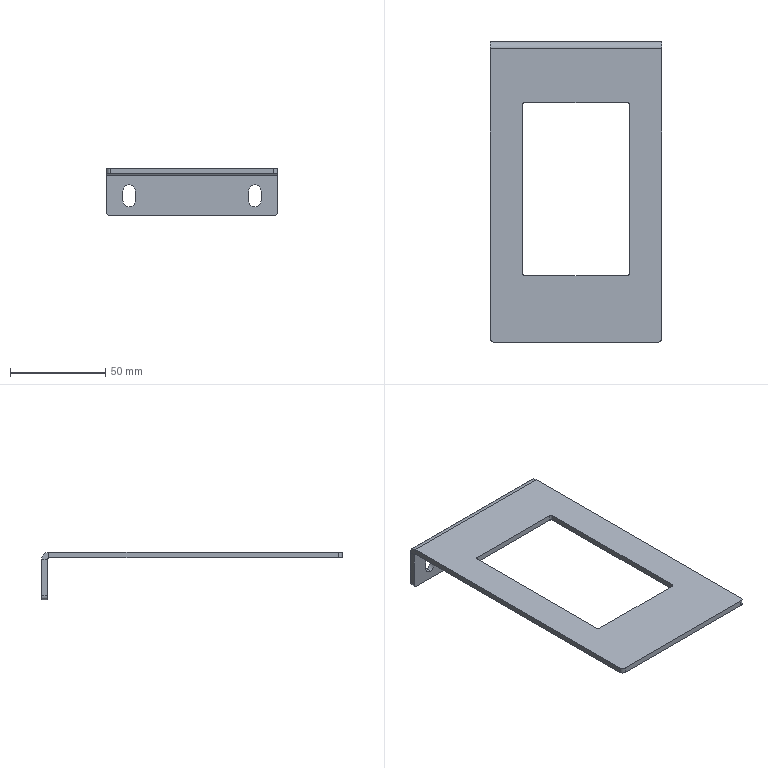Part | SolidWorks | features Fillet 2, ICE 2, EdgeFlange 1, FlatPattern 1, SMBaseFlange 1, SheetMetal 1 | 1 solid | 36 faces | box 90 x 158 x 25 mm | volume 32642 mm3 | plane 20 | cylinder 16 | commonest cylinder face diameters 6.6 x6 2 x4 4 x4 1.473 x1 7.473 x1
STEP:
#1=CARTESIAN_POINT('',(-33.,80.5,-20.3));
#2=VERTEX_POINT('',#1);
#3=CARTESIAN_POINT('',(-29.7,80.5,-17.));
#4=VERTEX_POINT('',#3);
#5=CARTESIAN_POINT('',(-33.,80.5,-17.));
#6=DIRECTION('',(0.,-1.,0.));
#7=DIRECTION('',(0.,0.,-1.));
#8=AXIS2_PLACEMENT_3D('',#5,#6,#7);
#9=CIRCLE('',#8,3.3);
#10=EDGE_CURVE('',#2,#4,#9,.T.);
#11=ORIENTED_EDGE('',*,*,#10,.F.);
#12=CARTESIAN_POINT('',(-33.,77.5,-20.3));
#13=VERTEX_POINT('',#12);
#14=CARTESIAN_POINT('',(-33.,80.5,-20.3));
#15=DIRECTION('',(0.,-1.,0.));
#16=VECTOR('',#15,1000.);
#17=LINE('',#14,#16);
#18=EDGE_CURVE('',#2,#13,#17,.T.);
#19=ORIENTED_EDGE('',*,*,#18,.T.);
#20=CARTESIAN_POINT('',(-29.7,77.5,-17.));
#21=VERTEX_POINT('',#20);
#22=CARTESIAN_POINT('',(-33.,77.5,-17.));
#23=DIRECTION('',(0.,-1.,0.));
#24=DIRECTION('',(0.,0.,-1.));
#25=AXIS2_PLACEMENT_3D('',#22,#23,#24);
#26=CIRCLE('',#25,3.3);
#27=EDGE_CURVE('',#13,#21,#26,.T.);
#28=ORIENTED_EDGE('',*,*,#27,.T.);
#29=CARTESIAN_POINT('',(-29.7,80.5,-17.));
#30=DIRECTION('',(0.,-1.,0.));
#31=VECTOR('',#30,1000.);
#32=LINE('',#29,#31);
#33=EDGE_CURVE('',#4,#21,#32,.T.);
#34=ORIENTED_EDGE('',*,*,#33,.F.);
#35=EDGE_LOOP('',(#11,#19,#28,#34));
#36=FACE_OUTER_BOUND('',#35,.T.);
#37=CARTESIAN_POINT('',(-33.,80.5,-17.));
#38=DIRECTION('',(0.,-1.,0.));
#39=DIRECTION('',(0.,0.,-1.));
#40=AXIS2_PLACEMENT_3D('',#37,#38,#39);
#41=CYLINDRICAL_SURFACE('',#40,3.3);
#42=ADVANCED_FACE('',(#36),#41,.F.);
#43=CARTESIAN_POINT('',(33.,80.5,-20.3));
#44=VERTEX_POINT('',#43);
#45=CARTESIAN_POINT('',(36.3,80.5,-17.));
#46=VERTEX_POINT('',#45);
#47=CARTESIAN_POINT('',(33.,80.5,-17.));
#48=DIRECTION('',(0.,-1.,0.));
#49=DIRECTION('',(0.,0.,-1.));
#50=AXIS2_PLACEMENT_3D('',#47,#48,#49);
#51=CIRCLE('',#50,3.3);
#52=EDGE_CURVE('',#44,#46,#51,.T.);
#53=ORIENTED_EDGE('',*,*,#52,.F.);
#54=CARTESIAN_POINT('',(33.,77.5,-20.3));
#55=VERTEX_POINT('',#54);
#56=CARTESIAN_POINT('',(33.,80.5,-20.3));
#57=DIRECTION('',(0.,-1.,0.));
#58=VECTOR('',#57,1000.);
#59=LINE('',#56,#58);
#60=EDGE_CURVE('',#44,#55,#59,.T.);
#61=ORIENTED_EDGE('',*,*,#60,.T.);
#62=CARTESIAN_POINT('',(36.3,77.5,-17.));
#63=VERTEX_POINT('',#62);
#64=CARTESIAN_POINT('',(33.,77.5,-17.));
#65=DIRECTION('',(0.,-1.,0.));
#66=DIRECTION('',(0.,0.,-1.));
#67=AXIS2_PLACEMENT_3D('',#64,#65,#66);
#68=CIRCLE('',#67,3.3);
#69=EDGE_CURVE('',#55,#63,#68,.T.);
#70=ORIENTED_EDGE('',*,*,#69,.T.);
#71=CARTESIAN_POINT('',(36.3,80.5,-17.));
#72=DIRECTION('',(0.,-1.,0.));
#73=VECTOR('',#72,1000.);
#74=LINE('',#71,#73);
#75=EDGE_CURVE('',#46,#63,#74,.T.);
#76=ORIENTED_EDGE('',*,*,#75,.F.);
#77=EDGE_LOOP('',(#53,#61,#70,#76));
#78=FACE_OUTER_BOUND('',#77,.T.);
#79=CARTESIAN_POINT('',(33.,80.5,-17.));
#80=DIRECTION('',(0.,-1.,0.));
#81=DIRECTION('',(0.,0.,-1.));
#82=AXIS2_PLACEMENT_3D('',#79,#80,#81);
#83=CYLINDRICAL_SURFACE('',#82,3.3);
#84=ADVANCED_FACE('',(#78),#83,.F.);
#85=CARTESIAN_POINT('',(45.,-75.5,0.));
#86=VERTEX_POINT('',#85);
#87=CARTESIAN_POINT('',(45.,76.763,0.));
#88=VERTEX_POINT('',#87);
#89=CARTESIAN_POINT('',(45.,77.5,0.));
#90=DIRECTION('',(0.,1.,0.));
#91=VECTOR('',#90,1000.);
#92=LINE('',#89,#91);
#93=EDGE_CURVE('',#86,#88,#92,.T.);
#94=ORIENTED_EDGE('',*,*,#93,.F.);
#95=CARTESIAN_POINT('',(45.,-75.5,-3.));
#96=VERTEX_POINT('',#95);
#97=CARTESIAN_POINT('',(45.,-75.5,-3.));
#98=DIRECTION('',(0.,0.,-1.));
#99=VECTOR('',#98,1000.);
#100=LINE('',#97,#99);
#101=EDGE_CURVE('',#86,#96,#100,.T.);
#102=ORIENTED_EDGE('',*,*,#101,.T.);
#103=CARTESIAN_POINT('',(45.,76.763,-3.));
#104=VERTEX_POINT('',#103);
#105=CARTESIAN_POINT('',(45.,77.5,-3.));
#106=DIRECTION('',(0.,1.,0.));
#107=VECTOR('',#106,1000.);
#108=LINE('',#105,#107);
#109=EDGE_CURVE('',#96,#104,#108,.T.);
#110=ORIENTED_EDGE('',*,*,#109,.T.);
#111=CARTESIAN_POINT('',(45.,76.763,-3.));
#112=DIRECTION('',(0.,0.,1.));
#113=VECTOR('',#112,1000.);
#114=LINE('',#111,#113);
#115=EDGE_CURVE('',#104,#88,#114,.T.);
#116=ORIENTED_EDGE('',*,*,#115,.T.);
#117=EDGE_LOOP('',(#94,#102,#110,#116));
#118=FACE_OUTER_BOUND('',#117,.T.);
#119=CARTESIAN_POINT('',(45.,77.5,-3.));
#120=DIRECTION('',(1.,0.,0.));
#121=DIRECTION('',(0.,1.,0.));
#122=AXIS2_PLACEMENT_3D('',#119,#120,#121);
#123=PLANE('',#122);
#124=ADVANCED_FACE('',(#118),#123,.T.);
#125=CARTESIAN_POINT('',(-27.,48.5,-3.));
#126=VERTEX_POINT('',#125);
#127=CARTESIAN_POINT('',(27.,48.5,-3.));
#128=VERTEX_POINT('',#127);
#129=CARTESIAN_POINT('',(28.,48.5,-3.));
#130=DIRECTION('',(1.,0.,0.));
#131=VECTOR('',#130,1000.);
#132=LINE('',#129,#131);
#133=EDGE_CURVE('',#126,#128,#132,.T.);
#134=ORIENTED_EDGE('',*,*,#133,.F.);
#135=CARTESIAN_POINT('',(-28.,47.5,-3.));
#136=VERTEX_POINT('',#135);
#137=CARTESIAN_POINT('',(-27.,47.5,-3.));
#138=DIRECTION('',(0.,0.,1.));
#139=DIRECTION('',(1.,0.,0.));
#140=AXIS2_PLACEMENT_3D('',#137,#138,#139);
#141=CIRCLE('',#140,1.);
#142=EDGE_CURVE('',#126,#136,#141,.T.);
#143=ORIENTED_EDGE('',*,*,#142,.T.);
#144=CARTESIAN_POINT('',(-28.,-41.5,-3.));
#145=VERTEX_POINT('',#144);
#146=CARTESIAN_POINT('',(-28.,-42.5,-3.));
#147=DIRECTION('',(0.,1.,0.));
#148=VECTOR('',#147,1000.);
#149=LINE('',#146,#148);
#150=EDGE_CURVE('',#145,#136,#149,.T.);
#151=ORIENTED_EDGE('',*,*,#150,.F.);
#152=CARTESIAN_POINT('',(-27.,-42.5,-3.));
#153=VERTEX_POINT('',#152);
#154=CARTESIAN_POINT('',(-27.,-41.5,-3.));
#155=DIRECTION('',(0.,0.,1.));
#156=DIRECTION('',(1.,0.,0.));
#157=AXIS2_PLACEMENT_3D('',#154,#155,#156);
#158=CIRCLE('',#157,1.);
#159=EDGE_CURVE('',#145,#153,#158,.T.);
#160=ORIENTED_EDGE('',*,*,#159,.T.);
#161=CARTESIAN_POINT('',(27.,-42.5,-3.));
#162=VERTEX_POINT('',#161);
#163=CARTESIAN_POINT('',(28.,-42.5,-3.));
#164=DIRECTION('',(-1.,0.,0.));
#165=VECTOR('',#164,1000.);
#166=LINE('',#163,#165);
#167=EDGE_CURVE('',#162,#153,#166,.T.);
#168=ORIENTED_EDGE('',*,*,#167,.F.);
#169=CARTESIAN_POINT('',(28.,-41.5,-3.));
#170=VERTEX_POINT('',#169);
#171=CARTESIAN_POINT('',(27.,-41.5,-3.));
#172=DIRECTION('',(0.,0.,1.));
#173=DIRECTION('',(1.,0.,0.));
#174=AXIS2_PLACEMENT_3D('',#171,#172,#173);
#175=CIRCLE('',#174,1.);
#176=EDGE_CURVE('',#162,#170,#175,.T.);
#177=ORIENTED_EDGE('',*,*,#176,.T.);
#178=CARTESIAN_POINT('',(28.,47.5,-3.));
#179=VERTEX_POINT('',#178);
#180=CARTESIAN_POINT('',(28.,-42.5,-3.));
#181=DIRECTION('',(0.,-1.,0.));
#182=VECTOR('',#181,1000.);
#183=LINE('',#180,#182);
#184=EDGE_CURVE('',#179,#170,#183,.T.);
#185=ORIENTED_EDGE('',*,*,#184,.F.);
#186=CARTESIAN_POINT('',(27.,47.5,-3.));
#187=DIRECTION('',(0.,0.,1.));
#188=DIRECTION('',(1.,0.,0.));
#189=AXIS2_PLACEMENT_3D('',#186,#187,#188);
#190=CIRCLE('',#189,1.);
#191=EDGE_CURVE('',#179,#128,#190,.T.);
#192=ORIENTED_EDGE('',*,*,#191,.T.);
#193=EDGE_LOOP('',(#134,#143,#151,#160,#168,#177,#185,#192));
#194=FACE_BOUND('',#193,.T.);
#195=CARTESIAN_POINT('',(-43.,-77.5,-3.));
#196=VERTEX_POINT('',#195);
#197=CARTESIAN_POINT('',(43.,-77.5,-3.));
#198=VERTEX_POINT('',#197);
#199=CARTESIAN_POINT('',(-45.,-77.5,-3.));
#200=DIRECTION('',(1.,0.,0.));
#201=VECTOR('',#200,1000.);
#202=LINE('',#199,#201);
#203=EDGE_CURVE('',#196,#198,#202,.T.);
#204=ORIENTED_EDGE('',*,*,#203,.F.);
#205=CARTESIAN_POINT('',(-45.,-75.5,-3.));
#206=VERTEX_POINT('',#205);
#207=CARTESIAN_POINT('',(-43.,-75.5,-3.));
#208=DIRECTION('',(0.,0.,-1.));
#209=DIRECTION('',(1.,0.,0.));
#210=AXIS2_PLACEMENT_3D('',#207,#208,#209);
#211=CIRCLE('',#210,2.);
#212=EDGE_CURVE('',#196,#206,#211,.T.);
#213=ORIENTED_EDGE('',*,*,#212,.T.);
#214=CARTESIAN_POINT('',(-45.,76.763,-3.));
#215=VERTEX_POINT('',#214);
#216=CARTESIAN_POINT('',(-45.,77.5,-3.));
#217=DIRECTION('',(0.,-1.,0.));
#218=VECTOR('',#217,1000.);
#219=LINE('',#216,#218);
#220=EDGE_CURVE('',#215,#206,#219,.T.);
#221=ORIENTED_EDGE('',*,*,#220,.F.);
#222=CARTESIAN_POINT('',(45.,76.763,-3.));
#223=DIRECTION('',(-1.,0.,0.));
#224=VECTOR('',#223,1000.);
#225=LINE('',#222,#224);
#226=EDGE_CURVE('',#104,#215,#225,.T.);
#227=ORIENTED_EDGE('',*,*,#226,.F.);
#228=ORIENTED_EDGE('',*,*,#109,.F.);
#229=CARTESIAN_POINT('',(43.,-75.5,-3.));
#230=DIRECTION('',(0.,0.,-1.));
#231=DIRECTION('',(1.,0.,0.));
#232=AXIS2_PLACEMENT_3D('',#229,#230,#231);
#233=CIRCLE('',#232,2.);
#234=EDGE_CURVE('',#96,#198,#233,.T.);
#235=ORIENTED_EDGE('',*,*,#234,.T.);
#236=EDGE_LOOP('',(#204,#213,#221,#227,#228,#235));
#237=FACE_OUTER_BOUND('',#236,.T.);
#238=CARTESIAN_POINT('',(45.,-77.5,-3.));
#239=DIRECTION('',(0.,0.,1.));
#240=DIRECTION('',(1.,0.,0.));
#241=AXIS2_PLACEMENT_3D('',#238,#239,#240);
#242=PLANE('',#241);
#243=ADVANCED_FACE('',(#194,#237),#242,.F.);
#244=CARTESIAN_POINT('',(27.,-42.5,0.));
#245=VERTEX_POINT('',#244);
#246=CARTESIAN_POINT('',(-27.,-42.5,0.));
#247=VERTEX_POINT('',#246);
#248=CARTESIAN_POINT('',(28.,-42.5,0.));
#249=DIRECTION('',(-1.,0.,0.));
#250=VECTOR('',#249,1000.);
#251=LINE('',#248,#250);
#252=EDGE_CURVE('',#245,#247,#251,.T.);
#253=ORIENTED_EDGE('',*,*,#252,.T.);
#254=CARTESIAN_POINT('',(-28.,-41.5,0.));
#255=VERTEX_POINT('',#254);
#256=CARTESIAN_POINT('',(-27.,-41.5,0.));
#257=DIRECTION('',(0.,0.,-1.));
#258=DIRECTION('',(1.,0.,0.));
#259=AXIS2_PLACEMENT_3D('',#256,#257,#258);
#260=CIRCLE('',#259,1.);
#261=EDGE_CURVE('',#247,#255,#260,.T.);
#262=ORIENTED_EDGE('',*,*,#261,.T.);
#263=CARTESIAN_POINT('',(-28.,47.5,0.));
#264=VERTEX_POINT('',#263);
#265=CARTESIAN_POINT('',(-28.,-42.5,0.));
#266=DIRECTION('',(0.,1.,0.));
#267=VECTOR('',#266,1000.);
#268=LINE('',#265,#267);
#269=EDGE_CURVE('',#255,#264,#268,.T.);
#270=ORIENTED_EDGE('',*,*,#269,.T.);
#271=CARTESIAN_POINT('',(-27.,48.5,0.));
#272=VERTEX_POINT('',#271);
#273=CARTESIAN_POINT('',(-27.,47.5,0.));
#274=DIRECTION('',(0.,0.,-1.));
#275=DIRECTION('',(1.,0.,0.));
#276=AXIS2_PLACEMENT_3D('',#273,#274,#275);
#277=CIRCLE('',#276,1.);
#278=EDGE_CURVE('',#264,#272,#277,.T.);
#279=ORIENTED_EDGE('',*,*,#278,.T.);
#280=CARTESIAN_POINT('',(27.,48.5,0.));
#281=VERTEX_POINT('',#280);
#282=CARTESIAN_POINT('',(28.,48.5,0.));
#283=DIRECTION('',(1.,0.,0.));
#284=VECTOR('',#283,1000.);
#285=LINE('',#282,#284);
#286=EDGE_CURVE('',#272,#281,#285,.T.);
#287=ORIENTED_EDGE('',*,*,#286,.T.);
#288=CARTESIAN_POINT('',(28.,47.5,0.));
#289=VERTEX_POINT('',#288);
#290=CARTESIAN_POINT('',(27.,47.5,0.));
#291=DIRECTION('',(0.,0.,-1.));
#292=DIRECTION('',(1.,0.,0.));
#293=AXIS2_PLACEMENT_3D('',#290,#291,#292);
#294=CIRCLE('',#293,1.);
#295=EDGE_CURVE('',#281,#289,#294,.T.);
#296=ORIENTED_EDGE('',*,*,#295,.T.);
#297=CARTESIAN_POINT('',(28.,-41.5,0.));
#298=VERTEX_POINT('',#297);
#299=CARTESIAN_POINT('',(28.,-42.5,0.));
#300=DIRECTION('',(0.,-1.,0.));
#301=VECTOR('',#300,1000.);
#302=LINE('',#299,#301);
#303=EDGE_CURVE('',#289,#298,#302,.T.);
#304=ORIENTED_EDGE('',*,*,#303,.T.);
#305=CARTESIAN_POINT('',(27.,-41.5,0.));
#306=DIRECTION('',(0.,0.,-1.));
#307=DIRECTION('',(1.,0.,0.));
#308=AXIS2_PLACEMENT_3D('',#305,#306,#307);
#309=CIRCLE('',#308,1.);
#310=EDGE_CURVE('',#298,#245,#309,.T.);
#311=ORIENTED_EDGE('',*,*,#310,.T.);
#312=EDGE_LOOP('',(#253,#262,#270,#279,#287,#296,#304,#311));
#313=FACE_BOUND('',#312,.T.);
#314=CARTESIAN_POINT('',(-45.,76.763,0.));
#315=VERTEX_POINT('',#314);
#316=CARTESIAN_POINT('',(-45.,-75.5,0.));
#317=VERTEX_POINT('',#316);
#318=CARTESIAN_POINT('',(-45.,77.5,0.));
#319=DIRECTION('',(0.,-1.,0.));
#320=VECTOR('',#319,1000.);
#321=LINE('',#318,#320);
#322=EDGE_CURVE('',#315,#317,#321,.T.);
#323=ORIENTED_EDGE('',*,*,#322,.T.);
#324=CARTESIAN_POINT('',(-43.,-77.5,0.));
#325=VERTEX_POINT('',#324);
#326=CARTESIAN_POINT('',(-43.,-75.5,0.));
#327=DIRECTION('',(0.,0.,1.));
#328=DIRECTION('',(1.,0.,0.));
#329=AXIS2_PLACEMENT_3D('',#326,#327,#328);
#330=CIRCLE('',#329,2.);
#331=EDGE_CURVE('',#317,#325,#330,.T.);
#332=ORIENTED_EDGE('',*,*,#331,.T.);
#333=CARTESIAN_POINT('',(43.,-77.5,0.));
#334=VERTEX_POINT('',#333);
#335=CARTESIAN_POINT('',(-45.,-77.5,0.));
#336=DIRECTION('',(1.,0.,0.));
#337=VECTOR('',#336,1000.);
#338=LINE('',#335,#337);
#339=EDGE_CURVE('',#325,#334,#338,.T.);
#340=ORIENTED_EDGE('',*,*,#339,.T.);
#341=CARTESIAN_POINT('',(43.,-75.5,0.));
#342=DIRECTION('',(0.,0.,1.));
#343=DIRECTION('',(1.,0.,0.));
#344=AXIS2_PLACEMENT_3D('',#341,#342,#343);
#345=CIRCLE('',#344,2.);
#346=EDGE_CURVE('',#334,#86,#345,.T.);
#347=ORIENTED_EDGE('',*,*,#346,.T.);
#348=ORIENTED_EDGE('',*,*,#93,.T.);
#349=CARTESIAN_POINT('',(45.,76.763,0.));
#350=DIRECTION('',(-1.,0.,0.));
#351=VECTOR('',#350,1000.);
#352=LINE('',#349,#351);
#353=EDGE_CURVE('',#88,#315,#352,.T.);
#354=ORIENTED_EDGE('',*,*,#353,.T.);
#355=EDGE_LOOP('',(#323,#332,#340,#347,#348,#354));
#356=FACE_OUTER_BOUND('',#355,.T.);
#357=CARTESIAN_POINT('',(45.,-77.5,0.));
#358=DIRECTION('',(0.,0.,1.));
#359=DIRECTION('',(1.,0.,0.));
#360=AXIS2_PLACEMENT_3D('',#357,#358,#359);
#361=PLANE('',#360);
#362=ADVANCED_FACE('',(#313,#356),#361,.T.);
#363=ORIENTED_EDGE('',*,*,#339,.F.);
#364=CARTESIAN_POINT('',(-43.,-77.5,-3.));
#365=DIRECTION('',(0.,0.,-1.));
#366=VECTOR('',#365,1000.);
#367=LINE('',#364,#366);
#368=EDGE_CURVE('',#325,#196,#367,.T.);
#369=ORIENTED_EDGE('',*,*,#368,.T.);
#370=ORIENTED_EDGE('',*,*,#203,.T.);
#371=CARTESIAN_POINT('',(43.,-77.5,-3.));
#372=DIRECTION('',(0.,0.,1.));
#373=VECTOR('',#372,1000.);
#374=LINE('',#371,#373);
#375=EDGE_CURVE('',#198,#334,#374,.T.);
#376=ORIENTED_EDGE('',*,*,#375,.T.);
#377=EDGE_LOOP('',(#363,#369,#370,#376));
#378=FACE_OUTER_BOUND('',#377,.T.);
#379=CARTESIAN_POINT('',(-45.,-77.5,-3.));
#380=DIRECTION('',(0.,-1.,0.));
#381=DIRECTION('',(0.,0.,-1.));
#382=AXIS2_PLACEMENT_3D('',#379,#380,#381);
#383=PLANE('',#382);
#384=ADVANCED_FACE('',(#378),#383,.T.);
#385=ORIENTED_EDGE('',*,*,#220,.T.);
#386=CARTESIAN_POINT('',(-45.,-75.5,-3.));
#387=DIRECTION('',(0.,0.,1.));
#388=VECTOR('',#387,1000.);
#389=LINE('',#386,#388);
#390=EDGE_CURVE('',#206,#317,#389,.T.);
#391=ORIENTED_EDGE('',*,*,#390,.T.);
#392=ORIENTED_EDGE('',*,*,#322,.F.);
#393=CARTESIAN_POINT('',(-45.,76.763,-3.));
#394=DIRECTION('',(0.,0.,1.));
#395=VECTOR('',#394,1000.);
#396=LINE('',#393,#395);
#397=EDGE_CURVE('',#215,#315,#396,.T.);
#398=ORIENTED_EDGE('',*,*,#397,.F.);
#399=EDGE_LOOP('',(#385,#391,#392,#398));
#400=FACE_OUTER_BOUND('',#399,.T.);
#401=CARTESIAN_POINT('',(-45.,77.5,-3.));
#402=DIRECTION('',(-1.,0.,0.));
#403=DIRECTION('',(0.,-1.,0.));
#404=AXIS2_PLACEMENT_3D('',#401,#402,#403);
#405=PLANE('',#404);
#406=ADVANCED_FACE('',(#400),#405,.T.);
#407=CARTESIAN_POINT('',(-45.,77.5,-3.737));
#408=VERTEX_POINT('',#407);
#409=CARTESIAN_POINT('',(-45.,80.5,-3.737));
#410=VERTEX_POINT('',#409);
#411=CARTESIAN_POINT('',(-45.,77.5,-3.737));
#412=DIRECTION('',(0.,1.,0.));
#413=VECTOR('',#412,1000.);
#414=LINE('',#411,#413);
#415=EDGE_CURVE('',#408,#410,#414,.T.);
#416=ORIENTED_EDGE('',*,*,#415,.F.);
#417=CARTESIAN_POINT('',(-45.,76.763,-3.737));
#418=DIRECTION('',(-1.,0.,0.));
#419=DIRECTION('',(0.,0.,-1.));
#420=AXIS2_PLACEMENT_3D('',#417,#418,#419);
#421=CIRCLE('',#420,0.7366);
#422=EDGE_CURVE('',#215,#408,#421,.T.);
#423=ORIENTED_EDGE('',*,*,#422,.F.);
#424=ORIENTED_EDGE('',*,*,#397,.T.);
#425=CARTESIAN_POINT('',(-45.,76.763,-3.737));
#426=DIRECTION('',(-1.,0.,0.));
#427=DIRECTION('',(0.,0.,-1.));
#428=AXIS2_PLACEMENT_3D('',#425,#426,#427);
#429=CIRCLE('',#428,3.737);
#430=EDGE_CURVE('',#315,#410,#429,.T.);
#431=ORIENTED_EDGE('',*,*,#430,.T.);
#432=EDGE_LOOP('',(#416,#423,#424,#431));
#433=FACE_OUTER_BOUND('',#432,.T.);
#434=CARTESIAN_POINT('',(-45.,76.763,-3.737));
#435=DIRECTION('',(-1.,0.,0.));
#436=DIRECTION('',(0.,0.,1.));
#437=AXIS2_PLACEMENT_3D('',#434,#435,#436);
#438=PLANE('',#437);
#439=ADVANCED_FACE('',(#433),#438,.T.);
#440=ORIENTED_EDGE('',*,*,#353,.F.);
#441=CARTESIAN_POINT('',(45.,80.5,-3.737));
#442=VERTEX_POINT('',#441);
#443=CARTESIAN_POINT('',(45.,76.763,-3.737));
#444=DIRECTION('',(1.,0.,0.));
#445=DIRECTION('',(0.,0.,-1.));
#446=AXIS2_PLACEMENT_3D('',#443,#444,#445);
#447=CIRCLE('',#446,3.737);
#448=EDGE_CURVE('',#442,#88,#447,.T.);
#449=ORIENTED_EDGE('',*,*,#448,.F.);
#450=CARTESIAN_POINT('',(45.,80.5,-3.737));
#451=DIRECTION('',(-1.,0.,0.));
#452=VECTOR('',#451,1000.);
#453=LINE('',#450,#452);
#454=EDGE_CURVE('',#442,#410,#453,.T.);
#455=ORIENTED_EDGE('',*,*,#454,.T.);
#456=ORIENTED_EDGE('',*,*,#430,.F.);
#457=EDGE_LOOP('',(#440,#449,#455,#456));
#458=FACE_OUTER_BOUND('',#457,.T.);
#459=CARTESIAN_POINT('',(45.,76.763,-3.737));
#460=DIRECTION('',(1.,0.,0.));
#461=DIRECTION('',(0.,1.,0.));
#462=AXIS2_PLACEMENT_3D('',#459,#460,#461);
#463=CYLINDRICAL_SURFACE('',#462,3.737);
#464=ADVANCED_FACE('',(#458),#463,.T.);
#465=CARTESIAN_POINT('',(45.,77.5,-3.737));
#466=VERTEX_POINT('',#465);
#467=CARTESIAN_POINT('',(45.,76.763,-3.737));
#468=DIRECTION('',(1.,0.,0.));
#469=DIRECTION('',(0.,0.,-1.));
#470=AXIS2_PLACEMENT_3D('',#467,#468,#469);
#471=CIRCLE('',#470,0.7366);
#472=EDGE_CURVE('',#466,#104,#471,.T.);
#473=ORIENTED_EDGE('',*,*,#472,.F.);
#474=CARTESIAN_POINT('',(45.,77.5,-3.737));
#475=DIRECTION('',(0.,1.,0.));
#476=VECTOR('',#475,1000.);
#477=LINE('',#474,#476);
#478=EDGE_CURVE('',#466,#442,#477,.T.);
#479=ORIENTED_EDGE('',*,*,#478,.T.);
#480=ORIENTED_EDGE('',*,*,#448,.T.);
#481=ORIENTED_EDGE('',*,*,#115,.F.);
#482=EDGE_LOOP('',(#473,#479,#480,#481));
#483=FACE_OUTER_BOUND('',#482,.T.);
#484=CARTESIAN_POINT('',(45.,76.763,-3.737));
#485=DIRECTION('',(-1.,0.,0.));
#486=DIRECTION('',(0.,0.,1.));
#487=AXIS2_PLACEMENT_3D('',#484,#485,#486);
#488=PLANE('',#487);
#489=ADVANCED_FACE('',(#483),#488,.F.);
#490=ORIENTED_EDGE('',*,*,#226,.T.);
#491=ORIENTED_EDGE('',*,*,#422,.T.);
#492=CARTESIAN_POINT('',(-45.,77.5,-3.737));
#493=DIRECTION('',(1.,0.,0.));
#494=VECTOR('',#493,1000.);
#495=LINE('',#492,#494);
#496=EDGE_CURVE('',#408,#466,#495,.T.);
#497=ORIENTED_EDGE('',*,*,#496,.T.);
#498=ORIENTED_EDGE('',*,*,#472,.T.);
#499=EDGE_LOOP('',(#490,#491,#497,#498));
#500=FACE_OUTER_BOUND('',#499,.T.);
#501=CARTESIAN_POINT('',(45.,76.763,-3.737));
#502=DIRECTION('',(1.,0.,0.));
#503=DIRECTION('',(0.,1.,0.));
#504=AXIS2_PLACEMENT_3D('',#501,#502,#503);
#505=CYLINDRICAL_SURFACE('',#504,0.7366);
#506=ADVANCED_FACE('',(#500),#505,.F.);
#507=CARTESIAN_POINT('',(45.,77.5,-23.));
#508=VERTEX_POINT('',#507);
#509=CARTESIAN_POINT('',(45.,77.5,-25.));
#510=DIRECTION('',(0.,0.,-1.));
#511=VECTOR('',#510,1000.);
#512=LINE('',#509,#511);
#513=EDGE_CURVE('',#466,#508,#512,.T.);
#514=ORIENTED_EDGE('',*,*,#513,.T.);
#515=CARTESIAN_POINT('',(45.,80.5,-23.));
#516=VERTEX_POINT('',#515);
#517=CARTESIAN_POINT('',(45.,80.5,-23.));
#518=DIRECTION('',(0.,1.,0.));
#519=VECTOR('',#518,1000.);
#520=LINE('',#517,#519);
#521=EDGE_CURVE('',#508,#516,#520,.T.);
#522=ORIENTED_EDGE('',*,*,#521,.T.);
#523=CARTESIAN_POINT('',(45.,80.5,-25.));
#524=DIRECTION('',(0.,0.,-1.));
#525=VECTOR('',#524,1000.);
#526=LINE('',#523,#525);
#527=EDGE_CURVE('',#442,#516,#526,.T.);
#528=ORIENTED_EDGE('',*,*,#527,.F.);
#529=ORIENTED_EDGE('',*,*,#478,.F.);
#530=EDGE_LOOP('',(#514,#522,#528,#529));
#531=FACE_OUTER_BOUND('',#530,.T.);
#532=CARTESIAN_POINT('',(45.,80.5,-25.));
#533=DIRECTION('',(-1.,0.,0.));
#534=DIRECTION('',(0.,0.,1.));
#535=AXIS2_PLACEMENT_3D('',#532,#533,#534);
#536=PLANE('',#535);
#537=ADVANCED_FACE('',(#531),#536,.F.);
#538=CARTESIAN_POINT('',(-45.,80.5,-23.));
#539=VERTEX_POINT('',#538);
#540=CARTESIAN_POINT('',(-45.,80.5,-3.));
#541=DIRECTION('',(0.,0.,1.));
#542=VECTOR('',#541,1000.);
#543=LINE('',#540,#542);
#544=EDGE_CURVE('',#539,#410,#543,.T.);
#545=ORIENTED_EDGE('',*,*,#544,.F.);
#546=CARTESIAN_POINT('',(-45.,77.5,-23.));
#547=VERTEX_POINT('',#546);
#548=CARTESIAN_POINT('',(-45.,80.5,-23.));
#549=DIRECTION('',(0.,-1.,0.));
#550=VECTOR('',#549,1000.);
#551=LINE('',#548,#550);
#552=EDGE_CURVE('',#539,#547,#551,.T.);
#553=ORIENTED_EDGE('',*,*,#552,.T.);
#554=CARTESIAN_POINT('',(-45.,77.5,-3.));
#555=DIRECTION('',(0.,0.,1.));
#556=VECTOR('',#555,1000.);
#557=LINE('',#554,#556);
#558=EDGE_CURVE('',#547,#408,#557,.T.);
#559=ORIENTED_EDGE('',*,*,#558,.T.);
#560=ORIENTED_EDGE('',*,*,#415,.T.);
#561=EDGE_LOOP('',(#545,#553,#559,#560));
#562=FACE_OUTER_BOUND('',#561,.T.);
#563=CARTESIAN_POINT('',(-45.,80.5,-3.));
#564=DIRECTION('',(1.,0.,0.));
#565=DIRECTION('',(0.,0.,-1.));
#566=AXIS2_PLACEMENT_3D('',#563,#564,#565);
#567=PLANE('',#566);
#568=ADVANCED_FACE('',(#562),#567,.F.);
#569=CARTESIAN_POINT('',(-36.3,80.5,-12.));
#570=VERTEX_POINT('',#569);
#571=CARTESIAN_POINT('',(-36.3,80.5,-17.));
#572=VERTEX_POINT('',#571);
#573=CARTESIAN_POINT('',(-36.3,80.5,-17.));
#574=DIRECTION('',(0.,0.,-1.));
#575=VECTOR('',#574,1000.);
#576=LINE('',#573,#575);
#577=EDGE_CURVE('',#570,#572,#576,.T.);
#578=ORIENTED_EDGE('',*,*,#577,.T.);
#579=CARTESIAN_POINT('',(-33.,80.5,-17.));
#580=DIRECTION('',(0.,-1.,0.));
#581=DIRECTION('',(0.,0.,-1.));
#582=AXIS2_PLACEMENT_3D('',#579,#580,#581);
#583=CIRCLE('',#582,3.3);
#584=EDGE_CURVE('',#572,#2,#583,.T.);
#585=ORIENTED_EDGE('',*,*,#584,.T.);
#586=ORIENTED_EDGE('',*,*,#10,.T.);
#587=CARTESIAN_POINT('',(-29.7,80.5,-12.));
#588=VERTEX_POINT('',#587);
#589=CARTESIAN_POINT('',(-29.7,80.5,-17.));
#590=DIRECTION('',(0.,0.,1.));
#591=VECTOR('',#590,1000.);
#592=LINE('',#589,#591);
#593=EDGE_CURVE('',#4,#588,#592,.T.);
#594=ORIENTED_EDGE('',*,*,#593,.T.);
#595=CARTESIAN_POINT('',(-33.,80.5,-12.));
#596=DIRECTION('',(0.,-1.,0.));
#597=DIRECTION('',(0.,0.,-1.));
#598=AXIS2_PLACEMENT_3D('',#595,#596,#597);
#599=CIRCLE('',#598,3.3);
#600=EDGE_CURVE('',#588,#570,#599,.T.);
#601=ORIENTED_EDGE('',*,*,#600,.T.);
#602=EDGE_LOOP('',(#578,#585,#586,#594,#601));
#603=FACE_BOUND('',#602,.T.);
#604=CARTESIAN_POINT('',(29.7,80.5,-12.));
#605=VERTEX_POINT('',#604);
#606=CARTESIAN_POINT('',(29.7,80.5,-17.));
#607=VERTEX_POINT('',#606);
#608=CARTESIAN_POINT('',(29.7,80.5,-17.));
#609=DIRECTION('',(0.,0.,-1.));
#610=VECTOR('',#609,1000.);
#611=LINE('',#608,#610);
#612=EDGE_CURVE('',#605,#607,#611,.T.);
#613=ORIENTED_EDGE('',*,*,#612,.T.);
#614=CARTESIAN_POINT('',(33.,80.5,-17.));
#615=DIRECTION('',(0.,-1.,0.));
#616=DIRECTION('',(0.,0.,-1.));
#617=AXIS2_PLACEMENT_3D('',#614,#615,#616);
#618=CIRCLE('',#617,3.3);
#619=EDGE_CURVE('',#607,#44,#618,.T.);
#620=ORIENTED_EDGE('',*,*,#619,.T.);
#621=ORIENTED_EDGE('',*,*,#52,.T.);
#622=CARTESIAN_POINT('',(36.3,80.5,-12.));
#623=VERTEX_POINT('',#622);
#624=CARTESIAN_POINT('',(36.3,80.5,-17.));
#625=DIRECTION('',(0.,0.,1.));
#626=VECTOR('',#625,1000.);
#627=LINE('',#624,#626);
#628=EDGE_CURVE('',#46,#623,#627,.T.);
#629=ORIENTED_EDGE('',*,*,#628,.T.);
#630=CARTESIAN_POINT('',(33.,80.5,-12.));
#631=DIRECTION('',(0.,-1.,0.));
#632=DIRECTION('',(0.,0.,-1.));
#633=AXIS2_PLACEMENT_3D('',#630,#631,#632);
#634=CIRCLE('',#633,3.3);
#635=EDGE_CURVE('',#623,#605,#634,.T.);
#636=ORIENTED_EDGE('',*,*,#635,.T.);
#637=EDGE_LOOP('',(#613,#620,#621,#629,#636));
#638=FACE_BOUND('',#637,.T.);
#639=CARTESIAN_POINT('',(43.,80.5,-25.));
#640=VERTEX_POINT('',#639);
#641=CARTESIAN_POINT('',(-43.,80.5,-25.));
#642=VERTEX_POINT('',#641);
#643=CARTESIAN_POINT('',(-45.,80.5,-25.));
#644=DIRECTION('',(-1.,0.,0.));
#645=VECTOR('',#644,1000.);
#646=LINE('',#643,#645);
#647=EDGE_CURVE('',#640,#642,#646,.T.);
#648=ORIENTED_EDGE('',*,*,#647,.T.);
#649=CARTESIAN_POINT('',(-43.,80.5,-23.));
#650=DIRECTION('',(0.,1.,0.));
#651=DIRECTION('',(0.,0.,-1.));
#652=AXIS2_PLACEMENT_3D('',#649,#650,#651);
#653=CIRCLE('',#652,2.);
#654=EDGE_CURVE('',#642,#539,#653,.T.);
#655=ORIENTED_EDGE('',*,*,#654,.T.);
#656=ORIENTED_EDGE('',*,*,#544,.T.);
#657=ORIENTED_EDGE('',*,*,#454,.F.);
#658=ORIENTED_EDGE('',*,*,#527,.T.);
#659=CARTESIAN_POINT('',(43.,80.5,-23.));
#660=DIRECTION('',(0.,1.,0.));
#661=DIRECTION('',(0.,0.,-1.));
#662=AXIS2_PLACEMENT_3D('',#659,#660,#661);
#663=CIRCLE('',#662,2.);
#664=EDGE_CURVE('',#516,#640,#663,.T.);
#665=ORIENTED_EDGE('',*,*,#664,.T.);
#666=EDGE_LOOP('',(#648,#655,#656,#657,#658,#665));
#667=FACE_OUTER_BOUND('',#666,.T.);
#668=CARTESIAN_POINT('',(45.,80.5,-3.));
#669=DIRECTION('',(0.,-1.,0.));
#670=DIRECTION('',(0.,0.,-1.));
#671=AXIS2_PLACEMENT_3D('',#668,#669,#670);
#672=PLANE('',#671);
#673=ADVANCED_FACE('',(#603,#638,#667),#672,.F.);
#674=CARTESIAN_POINT('',(-36.3,77.5,-17.));
#675=VERTEX_POINT('',#674);
#676=CARTESIAN_POINT('',(-33.,77.5,-17.));
#677=DIRECTION('',(0.,-1.,0.));
#678=DIRECTION('',(0.,0.,-1.));
#679=AXIS2_PLACEMENT_3D('',#676,#677,#678);
#680=CIRCLE('',#679,3.3);
#681=EDGE_CURVE('',#675,#13,#680,.T.);
#682=ORIENTED_EDGE('',*,*,#681,.F.);
#683=CARTESIAN_POINT('',(-36.3,77.5,-12.));
#684=VERTEX_POINT('',#683);
#685=CARTESIAN_POINT('',(-36.3,77.5,-17.));
#686=DIRECTION('',(0.,0.,-1.));
#687=VECTOR('',#686,1000.);
#688=LINE('',#685,#687);
#689=EDGE_CURVE('',#684,#675,#688,.T.);
#690=ORIENTED_EDGE('',*,*,#689,.F.);
#691=CARTESIAN_POINT('',(-29.7,77.5,-12.));
#692=VERTEX_POINT('',#691);
#693=CARTESIAN_POINT('',(-33.,77.5,-12.));
#694=DIRECTION('',(0.,-1.,0.));
#695=DIRECTION('',(0.,0.,-1.));
#696=AXIS2_PLACEMENT_3D('',#693,#694,#695);
#697=CIRCLE('',#696,3.3);
#698=EDGE_CURVE('',#692,#684,#697,.T.);
#699=ORIENTED_EDGE('',*,*,#698,.F.);
#700=CARTESIAN_POINT('',(-29.7,77.5,-17.));
#701=DIRECTION('',(0.,0.,1.));
#702=VECTOR('',#701,1000.);
#703=LINE('',#700,#702);
#704=EDGE_CURVE('',#21,#692,#703,.T.);
#705=ORIENTED_EDGE('',*,*,#704,.F.);
#706=ORIENTED_EDGE('',*,*,#27,.F.);
#707=EDGE_LOOP('',(#682,#690,#699,#705,#706));
#708=FACE_BOUND('',#707,.T.);
#709=CARTESIAN_POINT('',(29.7,77.5,-17.));
#710=VERTEX_POINT('',#709);
#711=CARTESIAN_POINT('',(33.,77.5,-17.));
#712=DIRECTION('',(0.,-1.,0.));
#713=DIRECTION('',(0.,0.,-1.));
#714=AXIS2_PLACEMENT_3D('',#711,#712,#713);
#715=CIRCLE('',#714,3.3);
#716=EDGE_CURVE('',#710,#55,#715,.T.);
#717=ORIENTED_EDGE('',*,*,#716,.F.);
#718=CARTESIAN_POINT('',(29.7,77.5,-12.));
#719=VERTEX_POINT('',#718);
#720=CARTESIAN_POINT('',(29.7,77.5,-17.));
#721=DIRECTION('',(0.,0.,-1.));
#722=VECTOR('',#721,1000.);
#723=LINE('',#720,#722);
#724=EDGE_CURVE('',#719,#710,#723,.T.);
#725=ORIENTED_EDGE('',*,*,#724,.F.);
#726=CARTESIAN_POINT('',(36.3,77.5,-12.));
#727=VERTEX_POINT('',#726);
#728=CARTESIAN_POINT('',(33.,77.5,-12.));
#729=DIRECTION('',(0.,-1.,0.));
#730=DIRECTION('',(0.,0.,-1.));
#731=AXIS2_PLACEMENT_3D('',#728,#729,#730);
#732=CIRCLE('',#731,3.3);
#733=EDGE_CURVE('',#727,#719,#732,.T.);
#734=ORIENTED_EDGE('',*,*,#733,.F.);
#735=CARTESIAN_POINT('',(36.3,77.5,-17.));
#736=DIRECTION('',(0.,0.,1.));
#737=VECTOR('',#736,1000.);
#738=LINE('',#735,#737);
#739=EDGE_CURVE('',#63,#727,#738,.T.);
#740=ORIENTED_EDGE('',*,*,#739,.F.);
#741=ORIENTED_EDGE('',*,*,#69,.F.);
#742=EDGE_LOOP('',(#717,#725,#734,#740,#741));
#743=FACE_BOUND('',#742,.T.);
#744=ORIENTED_EDGE('',*,*,#558,.F.);
#745=CARTESIAN_POINT('',(-43.,77.5,-25.));
#746=VERTEX_POINT('',#745);
#747=CARTESIAN_POINT('',(-43.,77.5,-23.));
#748=DIRECTION('',(0.,-1.,0.));
#749=DIRECTION('',(0.,0.,-1.));
#750=AXIS2_PLACEMENT_3D('',#747,#748,#749);
#751=CIRCLE('',#750,2.);
#752=EDGE_CURVE('',#547,#746,#751,.T.);
#753=ORIENTED_EDGE('',*,*,#752,.T.);
#754=CARTESIAN_POINT('',(43.,77.5,-25.));
#755=VERTEX_POINT('',#754);
#756=CARTESIAN_POINT('',(-45.,77.5,-25.));
#757=DIRECTION('',(-1.,0.,0.));
#758=VECTOR('',#757,1000.);
#759=LINE('',#756,#758);
#760=EDGE_CURVE('',#755,#746,#759,.T.);
#761=ORIENTED_EDGE('',*,*,#760,.F.);
#762=CARTESIAN_POINT('',(43.,77.5,-23.));
#763=DIRECTION('',(0.,-1.,0.));
#764=DIRECTION('',(0.,0.,-1.));
#765=AXIS2_PLACEMENT_3D('',#762,#763,#764);
#766=CIRCLE('',#765,2.);
#767=EDGE_CURVE('',#755,#508,#766,.T.);
#768=ORIENTED_EDGE('',*,*,#767,.T.);
#769=ORIENTED_EDGE('',*,*,#513,.F.);
#770=ORIENTED_EDGE('',*,*,#496,.F.);
#771=EDGE_LOOP('',(#744,#753,#761,#768,#769,#770));
#772=FACE_OUTER_BOUND('',#771,.T.);
#773=CARTESIAN_POINT('',(45.,77.5,-3.));
#774=DIRECTION('',(0.,-1.,0.));
#775=DIRECTION('',(0.,0.,-1.));
#776=AXIS2_PLACEMENT_3D('',#773,#774,#775);
#777=PLANE('',#776);
#778=ADVANCED_FACE('',(#708,#743,#772),#777,.T.);
#779=ORIENTED_EDGE('',*,*,#760,.T.);
#780=CARTESIAN_POINT('',(-43.,80.5,-25.));
#781=DIRECTION('',(0.,1.,0.));
#782=VECTOR('',#781,1000.);
#783=LINE('',#780,#782);
#784=EDGE_CURVE('',#746,#642,#783,.T.);
#785=ORIENTED_EDGE('',*,*,#784,.T.);
#786=ORIENTED_EDGE('',*,*,#647,.F.);
#787=CARTESIAN_POINT('',(43.,80.5,-25.));
#788=DIRECTION('',(0.,-1.,0.));
#789=VECTOR('',#788,1000.);
#790=LINE('',#787,#789);
#791=EDGE_CURVE('',#640,#755,#790,.T.);
#792=ORIENTED_EDGE('',*,*,#791,.T.);
#793=EDGE_LOOP('',(#779,#785,#786,#792));
#794=FACE_OUTER_BOUND('',#793,.T.);
#795=CARTESIAN_POINT('',(-45.,80.5,-25.));
#796=DIRECTION('',(0.,0.,1.));
#797=DIRECTION('',(0.,-1.,0.));
#798=AXIS2_PLACEMENT_3D('',#795,#796,#797);
#799=PLANE('',#798);
#800=ADVANCED_FACE('',(#794),#799,.F.);
#801=ORIENTED_EDGE('',*,*,#60,.F.);
#802=ORIENTED_EDGE('',*,*,#619,.F.);
#803=CARTESIAN_POINT('',(29.7,80.5,-17.));
#804=DIRECTION('',(0.,-1.,0.));
#805=VECTOR('',#804,1000.);
#806=LINE('',#803,#805);
#807=EDGE_CURVE('',#607,#710,#806,.T.);
#808=ORIENTED_EDGE('',*,*,#807,.T.);
#809=ORIENTED_EDGE('',*,*,#716,.T.);
#810=EDGE_LOOP('',(#801,#802,#808,#809));
#811=FACE_OUTER_BOUND('',#810,.T.);
#812=CARTESIAN_POINT('',(33.,80.5,-17.));
#813=DIRECTION('',(0.,-1.,0.));
#814=DIRECTION('',(0.,0.,-1.));
#815=AXIS2_PLACEMENT_3D('',#812,#813,#814);
#816=CYLINDRICAL_SURFACE('',#815,3.3);
#817=ADVANCED_FACE('',(#811),#816,.F.);
#818=ORIENTED_EDGE('',*,*,#724,.T.);
#819=ORIENTED_EDGE('',*,*,#807,.F.);
#820=ORIENTED_EDGE('',*,*,#612,.F.);
#821=CARTESIAN_POINT('',(29.7,80.5,-12.));
#822=DIRECTION('',(0.,-1.,0.));
#823=VECTOR('',#822,1000.);
#824=LINE('',#821,#823);
#825=EDGE_CURVE('',#605,#719,#824,.T.);
#826=ORIENTED_EDGE('',*,*,#825,.T.);
#827=EDGE_LOOP('',(#818,#819,#820,#826));
#828=FACE_OUTER_BOUND('',#827,.T.);
#829=CARTESIAN_POINT('',(29.7,80.5,-17.));
#830=DIRECTION('',(-1.,0.,0.));
#831=DIRECTION('',(0.,0.,1.));
#832=AXIS2_PLACEMENT_3D('',#829,#830,#831);
#833=PLANE('',#832);
#834=ADVANCED_FACE('',(#828),#833,.F.);
#835=ORIENTED_EDGE('',*,*,#733,.T.);
#836=ORIENTED_EDGE('',*,*,#825,.F.);
#837=ORIENTED_EDGE('',*,*,#635,.F.);
#838=CARTESIAN_POINT('',(36.3,80.5,-12.));
#839=DIRECTION('',(0.,-1.,0.));
#840=VECTOR('',#839,1000.);
#841=LINE('',#838,#840);
#842=EDGE_CURVE('',#623,#727,#841,.T.);
#843=ORIENTED_EDGE('',*,*,#842,.T.);
#844=EDGE_LOOP('',(#835,#836,#837,#843));
#845=FACE_OUTER_BOUND('',#844,.T.);
#846=CARTESIAN_POINT('',(33.,80.5,-12.));
#847=DIRECTION('',(0.,-1.,0.));
#848=DIRECTION('',(0.,0.,-1.));
#849=AXIS2_PLACEMENT_3D('',#846,#847,#848);
#850=CYLINDRICAL_SURFACE('',#849,3.3);
#851=ADVANCED_FACE('',(#845),#850,.F.);
#852=ORIENTED_EDGE('',*,*,#739,.T.);
#853=ORIENTED_EDGE('',*,*,#842,.F.);
#854=ORIENTED_EDGE('',*,*,#628,.F.);
#855=ORIENTED_EDGE('',*,*,#75,.T.);
#856=EDGE_LOOP('',(#852,#853,#854,#855));
#857=FACE_OUTER_BOUND('',#856,.T.);
#858=CARTESIAN_POINT('',(36.3,80.5,-17.));
#859=DIRECTION('',(1.,0.,0.));
#860=DIRECTION('',(0.,0.,-1.));
#861=AXIS2_PLACEMENT_3D('',#858,#859,#860);
#862=PLANE('',#861);
#863=ADVANCED_FACE('',(#857),#862,.F.);
#864=ORIENTED_EDGE('',*,*,#18,.F.);
#865=ORIENTED_EDGE('',*,*,#584,.F.);
#866=CARTESIAN_POINT('',(-36.3,80.5,-17.));
#867=DIRECTION('',(0.,-1.,0.));
#868=VECTOR('',#867,1000.);
#869=LINE('',#866,#868);
#870=EDGE_CURVE('',#572,#675,#869,.T.);
#871=ORIENTED_EDGE('',*,*,#870,.T.);
#872=ORIENTED_EDGE('',*,*,#681,.T.);
#873=EDGE_LOOP('',(#864,#865,#871,#872));
#874=FACE_OUTER_BOUND('',#873,.T.);
#875=CARTESIAN_POINT('',(-33.,80.5,-17.));
#876=DIRECTION('',(0.,-1.,0.));
#877=DIRECTION('',(0.,0.,-1.));
#878=AXIS2_PLACEMENT_3D('',#875,#876,#877);
#879=CYLINDRICAL_SURFACE('',#878,3.3);
#880=ADVANCED_FACE('',(#874),#879,.F.);
#881=ORIENTED_EDGE('',*,*,#689,.T.);
#882=ORIENTED_EDGE('',*,*,#870,.F.);
#883=ORIENTED_EDGE('',*,*,#577,.F.);
#884=CARTESIAN_POINT('',(-36.3,80.5,-12.));
#885=DIRECTION('',(0.,-1.,0.));
#886=VECTOR('',#885,1000.);
#887=LINE('',#884,#886);
#888=EDGE_CURVE('',#570,#684,#887,.T.);
#889=ORIENTED_EDGE('',*,*,#888,.T.);
#890=EDGE_LOOP('',(#881,#882,#883,#889));
#891=FACE_OUTER_BOUND('',#890,.T.);
#892=CARTESIAN_POINT('',(-36.3,80.5,-17.));
#893=DIRECTION('',(-1.,0.,0.));
#894=DIRECTION('',(0.,0.,1.));
#895=AXIS2_PLACEMENT_3D('',#892,#893,#894);
#896=PLANE('',#895);
#897=ADVANCED_FACE('',(#891),#896,.F.);
#898=ORIENTED_EDGE('',*,*,#698,.T.);
#899=ORIENTED_EDGE('',*,*,#888,.F.);
#900=ORIENTED_EDGE('',*,*,#600,.F.);
#901=CARTESIAN_POINT('',(-29.7,80.5,-12.));
#902=DIRECTION('',(0.,-1.,0.));
#903=VECTOR('',#902,1000.);
#904=LINE('',#901,#903);
#905=EDGE_CURVE('',#588,#692,#904,.T.);
#906=ORIENTED_EDGE('',*,*,#905,.T.);
#907=EDGE_LOOP('',(#898,#899,#900,#906));
#908=FACE_OUTER_BOUND('',#907,.T.);
#909=CARTESIAN_POINT('',(-33.,80.5,-12.));
#910=DIRECTION('',(0.,-1.,0.));
#911=DIRECTION('',(0.,0.,-1.));
#912=AXIS2_PLACEMENT_3D('',#909,#910,#911);
#913=CYLINDRICAL_SURFACE('',#912,3.3);
#914=ADVANCED_FACE('',(#908),#913,.F.);
#915=ORIENTED_EDGE('',*,*,#704,.T.);
#916=ORIENTED_EDGE('',*,*,#905,.F.);
#917=ORIENTED_EDGE('',*,*,#593,.F.);
#918=ORIENTED_EDGE('',*,*,#33,.T.);
#919=EDGE_LOOP('',(#915,#916,#917,#918));
#920=FACE_OUTER_BOUND('',#919,.T.);
#921=CARTESIAN_POINT('',(-29.7,80.5,-17.));
#922=DIRECTION('',(1.,0.,0.));
#923=DIRECTION('',(0.,0.,-1.));
#924=AXIS2_PLACEMENT_3D('',#921,#922,#923);
#925=PLANE('',#924);
#926=ADVANCED_FACE('',(#920),#925,.F.);
#927=ORIENTED_EDGE('',*,*,#269,.F.);
#928=CARTESIAN_POINT('',(-28.,-41.5,-3.));
#929=DIRECTION('',(0.,0.,-1.));
#930=VECTOR('',#929,1000.);
#931=LINE('',#928,#930);
#932=EDGE_CURVE('',#255,#145,#931,.T.);
#933=ORIENTED_EDGE('',*,*,#932,.T.);
#934=ORIENTED_EDGE('',*,*,#150,.T.);
#935=CARTESIAN_POINT('',(-28.,47.5,0.));
#936=DIRECTION('',(0.,0.,1.));
#937=VECTOR('',#936,1000.);
#938=LINE('',#935,#937);
#939=EDGE_CURVE('',#136,#264,#938,.T.);
#940=ORIENTED_EDGE('',*,*,#939,.T.);
#941=EDGE_LOOP('',(#927,#933,#934,#940));
#942=FACE_OUTER_BOUND('',#941,.T.);
#943=CARTESIAN_POINT('',(-28.,-42.5,0.));
#944=DIRECTION('',(-1.,0.,0.));
#945=DIRECTION('',(0.,0.,1.));
#946=AXIS2_PLACEMENT_3D('',#943,#944,#945);
#947=PLANE('',#946);
#948=ADVANCED_FACE('',(#942),#947,.F.);
#949=ORIENTED_EDGE('',*,*,#167,.T.);
#950=CARTESIAN_POINT('',(-27.,-42.5,0.));
#951=DIRECTION('',(0.,0.,1.));
#952=VECTOR('',#951,1000.);
#953=LINE('',#950,#952);
#954=EDGE_CURVE('',#153,#247,#953,.T.);
#955=ORIENTED_EDGE('',*,*,#954,.T.);
#956=ORIENTED_EDGE('',*,*,#252,.F.);
#957=CARTESIAN_POINT('',(27.,-42.5,-3.));
#958=DIRECTION('',(0.,0.,-1.));
#959=VECTOR('',#958,1000.);
#960=LINE('',#957,#959);
#961=EDGE_CURVE('',#245,#162,#960,.T.);
#962=ORIENTED_EDGE('',*,*,#961,.T.);
#963=EDGE_LOOP('',(#949,#955,#956,#962));
#964=FACE_OUTER_BOUND('',#963,.T.);
#965=CARTESIAN_POINT('',(28.,-42.5,0.));
#966=DIRECTION('',(0.,-1.,0.));
#967=DIRECTION('',(0.,0.,-1.));
#968=AXIS2_PLACEMENT_3D('',#965,#966,#967);
#969=PLANE('',#968);
#970=ADVANCED_FACE('',(#964),#969,.F.);
#971=ORIENTED_EDGE('',*,*,#184,.T.);
#972=CARTESIAN_POINT('',(28.,-41.5,0.));
#973=DIRECTION('',(0.,0.,1.));
#974=VECTOR('',#973,1000.);
#975=LINE('',#972,#974);
#976=EDGE_CURVE('',#170,#298,#975,.T.);
#977=ORIENTED_EDGE('',*,*,#976,.T.);
#978=ORIENTED_EDGE('',*,*,#303,.F.);
#979=CARTESIAN_POINT('',(28.,47.5,-3.));
#980=DIRECTION('',(0.,0.,-1.));
#981=VECTOR('',#980,1000.);
#982=LINE('',#979,#981);
#983=EDGE_CURVE('',#289,#179,#982,.T.);
#984=ORIENTED_EDGE('',*,*,#983,.T.);
#985=EDGE_LOOP('',(#971,#977,#978,#984));
#986=FACE_OUTER_BOUND('',#985,.T.);
#987=CARTESIAN_POINT('',(28.,-42.5,0.));
#988=DIRECTION('',(1.,0.,0.));
#989=DIRECTION('',(0.,0.,-1.));
#990=AXIS2_PLACEMENT_3D('',#987,#988,#989);
#991=PLANE('',#990);
#992=ADVANCED_FACE('',(#986),#991,.F.);
#993=ORIENTED_EDGE('',*,*,#133,.T.);
#994=CARTESIAN_POINT('',(27.,48.5,0.));
#995=DIRECTION('',(0.,0.,1.));
#996=VECTOR('',#995,1000.);
#997=LINE('',#994,#996);
#998=EDGE_CURVE('',#128,#281,#997,.T.);
#999=ORIENTED_EDGE('',*,*,#998,.T.);
#1000=ORIENTED_EDGE('',*,*,#286,.F.);
#1001=CARTESIAN_POINT('',(-27.,48.5,-3.));
#1002=DIRECTION('',(0.,0.,-1.));
#1003=VECTOR('',#1002,1000.);
#1004=LINE('',#1001,#1003);
#1005=EDGE_CURVE('',#272,#126,#1004,.T.);
#1006=ORIENTED_EDGE('',*,*,#1005,.T.);
#1007=EDGE_LOOP('',(#993,#999,#1000,#1006));
#1008=FACE_OUTER_BOUND('',#1007,.T.);
#1009=CARTESIAN_POINT('',(28.,48.5,0.));
#1010=DIRECTION('',(0.,1.,0.));
#1011=DIRECTION('',(0.,0.,1.));
#1012=AXIS2_PLACEMENT_3D('',#1009,#1010,#1011);
#1013=PLANE('',#1012);
#1014=ADVANCED_FACE('',(#1008),#1013,.F.);
#1015=ORIENTED_EDGE('',*,*,#654,.F.);
#1016=ORIENTED_EDGE('',*,*,#784,.F.);
#1017=ORIENTED_EDGE('',*,*,#752,.F.);
#1018=ORIENTED_EDGE('',*,*,#552,.F.);
#1019=EDGE_LOOP('',(#1015,#1016,#1017,#1018));
#1020=FACE_OUTER_BOUND('',#1019,.T.);
#1021=CARTESIAN_POINT('',(-43.,80.5,-23.));
#1022=DIRECTION('',(0.,-1.,0.));
#1023=DIRECTION('',(0.,0.,-1.));
#1024=AXIS2_PLACEMENT_3D('',#1021,#1022,#1023);
#1025=CYLINDRICAL_SURFACE('',#1024,2.);
#1026=ADVANCED_FACE('',(#1020),#1025,.T.);
#1027=ORIENTED_EDGE('',*,*,#212,.F.);
#1028=ORIENTED_EDGE('',*,*,#368,.F.);
#1029=ORIENTED_EDGE('',*,*,#331,.F.);
#1030=ORIENTED_EDGE('',*,*,#390,.F.);
#1031=EDGE_LOOP('',(#1027,#1028,#1029,#1030));
#1032=FACE_OUTER_BOUND('',#1031,.T.);
#1033=CARTESIAN_POINT('',(-43.,-75.5,-3.));
#1034=DIRECTION('',(0.,0.,1.));
#1035=DIRECTION('',(1.,0.,0.));
#1036=AXIS2_PLACEMENT_3D('',#1033,#1034,#1035);
#1037=CYLINDRICAL_SURFACE('',#1036,2.);
#1038=ADVANCED_FACE('',(#1032),#1037,.T.);
#1039=ORIENTED_EDGE('',*,*,#234,.F.);
#1040=ORIENTED_EDGE('',*,*,#101,.F.);
#1041=ORIENTED_EDGE('',*,*,#346,.F.);
#1042=ORIENTED_EDGE('',*,*,#375,.F.);
#1043=EDGE_LOOP('',(#1039,#1040,#1041,#1042));
#1044=FACE_OUTER_BOUND('',#1043,.T.);
#1045=CARTESIAN_POINT('',(43.,-75.5,-3.));
#1046=DIRECTION('',(0.,0.,1.));
#1047=DIRECTION('',(1.,0.,0.));
#1048=AXIS2_PLACEMENT_3D('',#1045,#1046,#1047);
#1049=CYLINDRICAL_SURFACE('',#1048,2.);
#1050=ADVANCED_FACE('',(#1044),#1049,.T.);
#1051=ORIENTED_EDGE('',*,*,#664,.F.);
#1052=ORIENTED_EDGE('',*,*,#521,.F.);
#1053=ORIENTED_EDGE('',*,*,#767,.F.);
#1054=ORIENTED_EDGE('',*,*,#791,.F.);
#1055=EDGE_LOOP('',(#1051,#1052,#1053,#1054));
#1056=FACE_OUTER_BOUND('',#1055,.T.);
#1057=CARTESIAN_POINT('',(43.,80.5,-23.));
#1058=DIRECTION('',(0.,-1.,0.));
#1059=DIRECTION('',(0.,0.,-1.));
#1060=AXIS2_PLACEMENT_3D('',#1057,#1058,#1059);
#1061=CYLINDRICAL_SURFACE('',#1060,2.);
#1062=ADVANCED_FACE('',(#1056),#1061,.T.);
#1063=ORIENTED_EDGE('',*,*,#261,.F.);
#1064=ORIENTED_EDGE('',*,*,#954,.F.);
#1065=ORIENTED_EDGE('',*,*,#159,.F.);
#1066=ORIENTED_EDGE('',*,*,#932,.F.);
#1067=EDGE_LOOP('',(#1063,#1064,#1065,#1066));
#1068=FACE_OUTER_BOUND('',#1067,.T.);
#1069=CARTESIAN_POINT('',(-27.,-41.5,0.));
#1070=DIRECTION('',(0.,0.,1.));
#1071=DIRECTION('',(1.,0.,0.));
#1072=AXIS2_PLACEMENT_3D('',#1069,#1070,#1071);
#1073=CYLINDRICAL_SURFACE('',#1072,1.);
#1074=ADVANCED_FACE('',(#1068),#1073,.F.);
#1075=ORIENTED_EDGE('',*,*,#310,.F.);
#1076=ORIENTED_EDGE('',*,*,#976,.F.);
#1077=ORIENTED_EDGE('',*,*,#176,.F.);
#1078=ORIENTED_EDGE('',*,*,#961,.F.);
#1079=EDGE_LOOP('',(#1075,#1076,#1077,#1078));
#1080=FACE_OUTER_BOUND('',#1079,.T.);
#1081=CARTESIAN_POINT('',(27.,-41.5,0.));
#1082=DIRECTION('',(0.,0.,1.));
#1083=DIRECTION('',(1.,0.,0.));
#1084=AXIS2_PLACEMENT_3D('',#1081,#1082,#1083);
#1085=CYLINDRICAL_SURFACE('',#1084,1.);
#1086=ADVANCED_FACE('',(#1080),#1085,.F.);
#1087=ORIENTED_EDGE('',*,*,#295,.F.);
#1088=ORIENTED_EDGE('',*,*,#998,.F.);
#1089=ORIENTED_EDGE('',*,*,#191,.F.);
#1090=ORIENTED_EDGE('',*,*,#983,.F.);
#1091=EDGE_LOOP('',(#1087,#1088,#1089,#1090));
#1092=FACE_OUTER_BOUND('',#1091,.T.);
#1093=CARTESIAN_POINT('',(27.,47.5,0.));
#1094=DIRECTION('',(0.,0.,1.));
#1095=DIRECTION('',(1.,0.,0.));
#1096=AXIS2_PLACEMENT_3D('',#1093,#1094,#1095);
#1097=CYLINDRICAL_SURFACE('',#1096,1.);
#1098=ADVANCED_FACE('',(#1092),#1097,.F.);
#1099=ORIENTED_EDGE('',*,*,#278,.F.);
#1100=ORIENTED_EDGE('',*,*,#939,.F.);
#1101=ORIENTED_EDGE('',*,*,#142,.F.);
#1102=ORIENTED_EDGE('',*,*,#1005,.F.);
#1103=EDGE_LOOP('',(#1099,#1100,#1101,#1102));
#1104=FACE_OUTER_BOUND('',#1103,.T.);
#1105=CARTESIAN_POINT('',(-27.,47.5,0.));
#1106=DIRECTION('',(0.,0.,1.));
#1107=DIRECTION('',(1.,0.,0.));
#1108=AXIS2_PLACEMENT_3D('',#1105,#1106,#1107);
#1109=CYLINDRICAL_SURFACE('',#1108,1.);
#1110=ADVANCED_FACE('',(#1104),#1109,.F.);
#1111=CLOSED_SHELL('',(#42,#84,#124,#243,#362,#384,#406,#439,#464,#489,#506,#537,#568,#673,#778,#800,#817,#834,#851,#863,#880,#897,#914,#926,#948,#970,#992,#1014,#1026,#1038,#1050,#1062,#1074,#1086,#1098,#1110));
#1112=MANIFOLD_SOLID_BREP('',#1111);
#1113=CARTESIAN_POINT('',(0.,0.,0.));
#1114=DIRECTION('',(0.,0.,1.));
#1115=DIRECTION('',(1.,0.,0.));
#1116=AXIS2_PLACEMENT_3D('',#1113,#1114,#1115);
#1117=(LENGTH_UNIT()NAMED_UNIT(*)SI_UNIT(.MILLI.,.METRE.));
#1118=UNCERTAINTY_MEASURE_WITH_UNIT(LENGTH_MEASURE(0.00001),#1117,'','');
#1119=(NAMED_UNIT(*)PLANE_ANGLE_UNIT()SI_UNIT($,.RADIAN.));
#1120=(NAMED_UNIT(*)SI_UNIT($,.STERADIAN.)SOLID_ANGLE_UNIT());
#1121=(GEOMETRIC_REPRESENTATION_CONTEXT(3)GLOBAL_UNCERTAINTY_ASSIGNED_CONTEXT((#1118))GLOBAL_UNIT_ASSIGNED_CONTEXT((#1117,#1119,#1120))REPRESENTATION_CONTEXT('',''));
#1122=ADVANCED_BREP_SHAPE_REPRESENTATION('',(#1112,#1116),#1121);